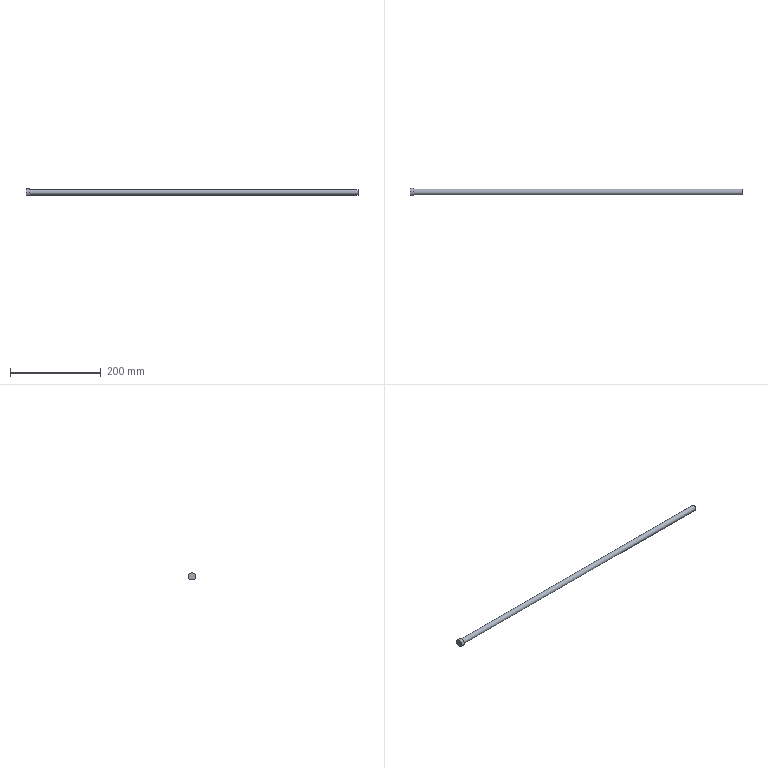Part | STEP file | solid 32 | 1 solid | 6 faces | box 730 x 17 x 15 mm | volume 83352 mm3 | plane 4 | cylinder 2 | commonest cylinder face diameters 12 x1 17 x1